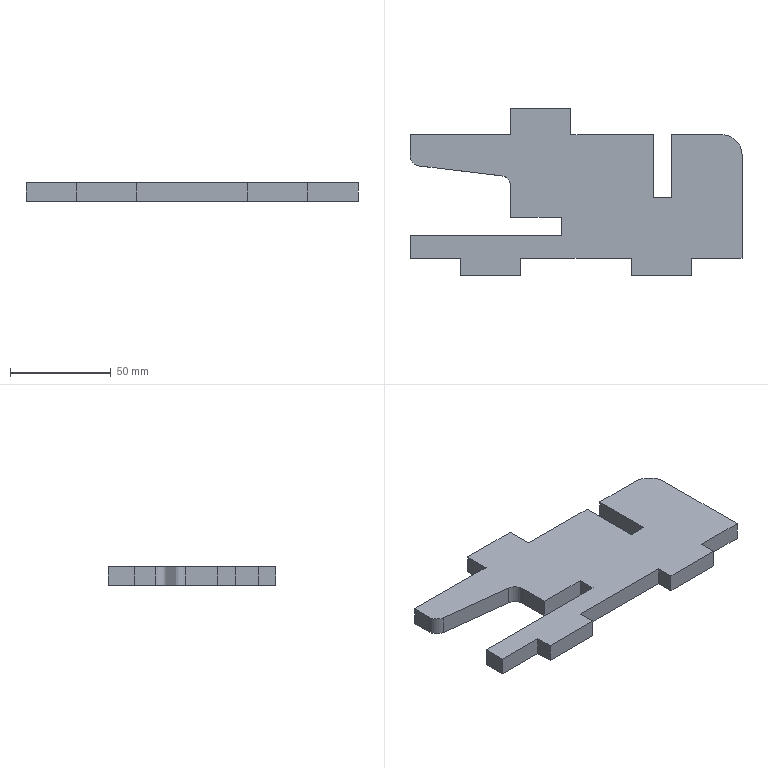Part | SolidWorks | features FlatPattern 1, SMBaseFlange 1, SheetMetal 1 | 1 solid | 31 faces | box 165 x 83 x 9 mm | volume 80282 mm3 | plane 28 | cylinder 3 | commonest cylinder face diameters 10 x2 20 x1
STEP:
#1=CARTESIAN_POINT('',(827.75,-98.803,0.));
#2=VERTEX_POINT('',#1);
#3=CARTESIAN_POINT('',(827.75,-110.303,0.));
#4=VERTEX_POINT('',#3);
#5=CARTESIAN_POINT('',(827.75,-110.303,0.));
#6=DIRECTION('',(0.,-1.,0.));
#7=VECTOR('',#6,1000.);
#8=LINE('',#5,#7);
#9=EDGE_CURVE('',#2,#4,#8,.T.);
#10=ORIENTED_EDGE('',*,*,#9,.F.);
#11=CARTESIAN_POINT('',(827.75,-98.803,-9.));
#12=VERTEX_POINT('',#11);
#13=CARTESIAN_POINT('',(827.75,-98.803,-9.));
#14=DIRECTION('',(0.,0.,1.));
#15=VECTOR('',#14,1000.);
#16=LINE('',#13,#15);
#17=EDGE_CURVE('',#12,#2,#16,.T.);
#18=ORIENTED_EDGE('',*,*,#17,.F.);
#19=CARTESIAN_POINT('',(827.75,-110.303,-9.));
#20=VERTEX_POINT('',#19);
#21=CARTESIAN_POINT('',(827.75,-110.303,-9.));
#22=DIRECTION('',(0.,-1.,0.));
#23=VECTOR('',#22,1000.);
#24=LINE('',#21,#23);
#25=EDGE_CURVE('',#12,#20,#24,.T.);
#26=ORIENTED_EDGE('',*,*,#25,.T.);
#27=CARTESIAN_POINT('',(827.75,-110.303,-9.));
#28=DIRECTION('',(0.,0.,1.));
#29=VECTOR('',#28,1000.);
#30=LINE('',#27,#29);
#31=EDGE_CURVE('',#20,#4,#30,.T.);
#32=ORIENTED_EDGE('',*,*,#31,.T.);
#33=EDGE_LOOP('',(#10,#18,#26,#32));
#34=FACE_OUTER_BOUND('',#33,.T.);
#35=CARTESIAN_POINT('',(827.75,-110.303,-9.));
#36=DIRECTION('',(-1.,0.,0.));
#37=DIRECTION('',(0.,-1.,0.));
#38=AXIS2_PLACEMENT_3D('',#35,#36,#37);
#39=PLANE('',#38);
#40=ADVANCED_FACE('',(#34),#39,.T.);
#41=CARTESIAN_POINT('',(902.95,-98.803,0.));
#42=VERTEX_POINT('',#41);
#43=CARTESIAN_POINT('',(827.75,-98.803,0.));
#44=DIRECTION('',(-1.,0.,0.));
#45=VECTOR('',#44,1000.);
#46=LINE('',#43,#45);
#47=EDGE_CURVE('',#42,#2,#46,.T.);
#48=ORIENTED_EDGE('',*,*,#47,.F.);
#49=CARTESIAN_POINT('',(902.95,-98.803,-9.));
#50=VERTEX_POINT('',#49);
#51=CARTESIAN_POINT('',(902.95,-98.803,-9.));
#52=DIRECTION('',(0.,0.,1.));
#53=VECTOR('',#52,1000.);
#54=LINE('',#51,#53);
#55=EDGE_CURVE('',#50,#42,#54,.T.);
#56=ORIENTED_EDGE('',*,*,#55,.F.);
#57=CARTESIAN_POINT('',(827.75,-98.803,-9.));
#58=DIRECTION('',(-1.,0.,0.));
#59=VECTOR('',#58,1000.);
#60=LINE('',#57,#59);
#61=EDGE_CURVE('',#50,#12,#60,.T.);
#62=ORIENTED_EDGE('',*,*,#61,.T.);
#63=ORIENTED_EDGE('',*,*,#17,.T.);
#64=EDGE_LOOP('',(#48,#56,#62,#63));
#65=FACE_OUTER_BOUND('',#64,.T.);
#66=CARTESIAN_POINT('',(827.75,-98.803,-9.));
#67=DIRECTION('',(0.,1.,0.));
#68=DIRECTION('',(0.,0.,1.));
#69=AXIS2_PLACEMENT_3D('',#66,#67,#68);
#70=PLANE('',#69);
#71=ADVANCED_FACE('',(#65),#70,.T.);
#72=CARTESIAN_POINT('',(902.95,-89.803,0.));
#73=VERTEX_POINT('',#72);
#74=CARTESIAN_POINT('',(902.95,-89.803,0.));
#75=DIRECTION('',(0.,-1.,0.));
#76=VECTOR('',#75,1000.);
#77=LINE('',#74,#76);
#78=EDGE_CURVE('',#73,#42,#77,.T.);
#79=ORIENTED_EDGE('',*,*,#78,.F.);
#80=CARTESIAN_POINT('',(902.95,-89.803,-9.));
#81=VERTEX_POINT('',#80);
#82=CARTESIAN_POINT('',(902.95,-89.803,-9.));
#83=DIRECTION('',(0.,0.,1.));
#84=VECTOR('',#83,1000.);
#85=LINE('',#82,#84);
#86=EDGE_CURVE('',#81,#73,#85,.T.);
#87=ORIENTED_EDGE('',*,*,#86,.F.);
#88=CARTESIAN_POINT('',(902.95,-89.803,-9.));
#89=DIRECTION('',(0.,-1.,0.));
#90=VECTOR('',#89,1000.);
#91=LINE('',#88,#90);
#92=EDGE_CURVE('',#81,#50,#91,.T.);
#93=ORIENTED_EDGE('',*,*,#92,.T.);
#94=ORIENTED_EDGE('',*,*,#55,.T.);
#95=EDGE_LOOP('',(#79,#87,#93,#94));
#96=FACE_OUTER_BOUND('',#95,.T.);
#97=CARTESIAN_POINT('',(902.95,-89.803,-9.));
#98=DIRECTION('',(-1.,0.,0.));
#99=DIRECTION('',(0.,0.,1.));
#100=AXIS2_PLACEMENT_3D('',#97,#98,#99);
#101=PLANE('',#100);
#102=ADVANCED_FACE('',(#96),#101,.T.);
#103=CARTESIAN_POINT('',(877.75,-89.803,0.));
#104=VERTEX_POINT('',#103);
#105=CARTESIAN_POINT('',(877.75,-89.803,0.));
#106=DIRECTION('',(1.,0.,0.));
#107=VECTOR('',#106,1000.);
#108=LINE('',#105,#107);
#109=EDGE_CURVE('',#104,#73,#108,.T.);
#110=ORIENTED_EDGE('',*,*,#109,.F.);
#111=CARTESIAN_POINT('',(877.75,-89.803,-9.));
#112=VERTEX_POINT('',#111);
#113=CARTESIAN_POINT('',(877.75,-89.803,-9.));
#114=DIRECTION('',(0.,0.,1.));
#115=VECTOR('',#114,1000.);
#116=LINE('',#113,#115);
#117=EDGE_CURVE('',#112,#104,#116,.T.);
#118=ORIENTED_EDGE('',*,*,#117,.F.);
#119=CARTESIAN_POINT('',(877.75,-89.803,-9.));
#120=DIRECTION('',(1.,0.,0.));
#121=VECTOR('',#120,1000.);
#122=LINE('',#119,#121);
#123=EDGE_CURVE('',#112,#81,#122,.T.);
#124=ORIENTED_EDGE('',*,*,#123,.T.);
#125=ORIENTED_EDGE('',*,*,#86,.T.);
#126=EDGE_LOOP('',(#110,#118,#124,#125));
#127=FACE_OUTER_BOUND('',#126,.T.);
#128=CARTESIAN_POINT('',(877.75,-89.803,-9.));
#129=DIRECTION('',(0.,-1.,0.));
#130=DIRECTION('',(1.,0.,0.));
#131=AXIS2_PLACEMENT_3D('',#128,#129,#130);
#132=PLANE('',#131);
#133=ADVANCED_FACE('',(#127),#132,.T.);
#134=CARTESIAN_POINT('',(877.75,-74.239,0.));
#135=VERTEX_POINT('',#134);
#136=CARTESIAN_POINT('',(877.75,-89.803,0.));
#137=DIRECTION('',(0.,-1.,0.));
#138=VECTOR('',#137,1000.);
#139=LINE('',#136,#138);
#140=EDGE_CURVE('',#135,#104,#139,.T.);
#141=ORIENTED_EDGE('',*,*,#140,.F.);
#142=CARTESIAN_POINT('',(877.75,-74.239,-9.));
#143=VERTEX_POINT('',#142);
#144=CARTESIAN_POINT('',(877.75,-74.239,-9.));
#145=DIRECTION('',(0.,0.,1.));
#146=VECTOR('',#145,1000.);
#147=LINE('',#144,#146);
#148=EDGE_CURVE('',#143,#135,#147,.T.);
#149=ORIENTED_EDGE('',*,*,#148,.F.);
#150=CARTESIAN_POINT('',(877.75,-89.803,-9.));
#151=DIRECTION('',(0.,-1.,0.));
#152=VECTOR('',#151,1000.);
#153=LINE('',#150,#152);
#154=EDGE_CURVE('',#143,#112,#153,.T.);
#155=ORIENTED_EDGE('',*,*,#154,.T.);
#156=ORIENTED_EDGE('',*,*,#117,.T.);
#157=EDGE_LOOP('',(#141,#149,#155,#156));
#158=FACE_OUTER_BOUND('',#157,.T.);
#159=CARTESIAN_POINT('',(877.75,-89.803,-9.));
#160=DIRECTION('',(-1.,0.,0.));
#161=DIRECTION('',(0.,-1.,0.));
#162=AXIS2_PLACEMENT_3D('',#159,#160,#161);
#163=PLANE('',#162);
#164=ADVANCED_FACE('',(#158),#163,.T.);
#165=CARTESIAN_POINT('',(873.346,-69.275,0.));
#166=VERTEX_POINT('',#165);
#167=CARTESIAN_POINT('',(872.75,-74.239,0.));
#168=DIRECTION('',(0.,0.,-1.));
#169=DIRECTION('',(1.,0.,0.));
#170=AXIS2_PLACEMENT_3D('',#167,#168,#169);
#171=CIRCLE('',#170,5.);
#172=EDGE_CURVE('',#166,#135,#171,.T.);
#173=ORIENTED_EDGE('',*,*,#172,.F.);
#174=CARTESIAN_POINT('',(873.346,-69.275,-9.));
#175=VERTEX_POINT('',#174);
#176=CARTESIAN_POINT('',(873.346,-69.275,-9.));
#177=DIRECTION('',(0.,0.,1.));
#178=VECTOR('',#177,1000.);
#179=LINE('',#176,#178);
#180=EDGE_CURVE('',#175,#166,#179,.T.);
#181=ORIENTED_EDGE('',*,*,#180,.F.);
#182=CARTESIAN_POINT('',(872.75,-74.239,-9.));
#183=DIRECTION('',(0.,0.,-1.));
#184=DIRECTION('',(1.,0.,0.));
#185=AXIS2_PLACEMENT_3D('',#182,#183,#184);
#186=CIRCLE('',#185,5.);
#187=EDGE_CURVE('',#175,#143,#186,.T.);
#188=ORIENTED_EDGE('',*,*,#187,.T.);
#189=ORIENTED_EDGE('',*,*,#148,.T.);
#190=EDGE_LOOP('',(#173,#181,#188,#189));
#191=FACE_OUTER_BOUND('',#190,.T.);
#192=CARTESIAN_POINT('',(872.75,-74.239,-9.));
#193=DIRECTION('',(0.,0.,1.));
#194=DIRECTION('',(1.,0.,0.));
#195=AXIS2_PLACEMENT_3D('',#192,#193,#194);
#196=CYLINDRICAL_SURFACE('',#195,5.);
#197=ADVANCED_FACE('',(#191),#196,.F.);
#198=CARTESIAN_POINT('',(832.154,-64.332,0.));
#199=VERTEX_POINT('',#198);
#200=CARTESIAN_POINT('',(873.346,-69.275,0.));
#201=DIRECTION('',(0.9929,-0.1191,0.));
#202=VECTOR('',#201,1000.);
#203=LINE('',#200,#202);
#204=EDGE_CURVE('',#199,#166,#203,.T.);
#205=ORIENTED_EDGE('',*,*,#204,.F.);
#206=CARTESIAN_POINT('',(832.154,-64.332,-9.));
#207=VERTEX_POINT('',#206);
#208=CARTESIAN_POINT('',(832.154,-64.332,-9.));
#209=DIRECTION('',(0.,0.,1.));
#210=VECTOR('',#209,1000.);
#211=LINE('',#208,#210);
#212=EDGE_CURVE('',#207,#199,#211,.T.);
#213=ORIENTED_EDGE('',*,*,#212,.F.);
#214=CARTESIAN_POINT('',(873.346,-69.275,-9.));
#215=DIRECTION('',(0.9929,-0.1191,0.));
#216=VECTOR('',#215,1000.);
#217=LINE('',#214,#216);
#218=EDGE_CURVE('',#207,#175,#217,.T.);
#219=ORIENTED_EDGE('',*,*,#218,.T.);
#220=ORIENTED_EDGE('',*,*,#180,.T.);
#221=EDGE_LOOP('',(#205,#213,#219,#220));
#222=FACE_OUTER_BOUND('',#221,.T.);
#223=CARTESIAN_POINT('',(873.346,-69.275,-9.));
#224=DIRECTION('',(-0.1191,-0.9929,0.));
#225=DIRECTION('',(0.9929,-0.1191,0.));
#226=AXIS2_PLACEMENT_3D('',#223,#224,#225);
#227=PLANE('',#226);
#228=ADVANCED_FACE('',(#222),#227,.T.);
#229=CARTESIAN_POINT('',(827.75,-59.367,0.));
#230=VERTEX_POINT('',#229);
#231=CARTESIAN_POINT('',(832.75,-59.367,0.));
#232=DIRECTION('',(0.,0.,1.));
#233=DIRECTION('',(-1.,0.,0.));
#234=AXIS2_PLACEMENT_3D('',#231,#232,#233);
#235=CIRCLE('',#234,5.);
#236=EDGE_CURVE('',#230,#199,#235,.T.);
#237=ORIENTED_EDGE('',*,*,#236,.F.);
#238=CARTESIAN_POINT('',(827.75,-59.367,-9.));
#239=VERTEX_POINT('',#238);
#240=CARTESIAN_POINT('',(827.75,-59.367,-9.));
#241=DIRECTION('',(0.,0.,1.));
#242=VECTOR('',#241,1000.);
#243=LINE('',#240,#242);
#244=EDGE_CURVE('',#239,#230,#243,.T.);
#245=ORIENTED_EDGE('',*,*,#244,.F.);
#246=CARTESIAN_POINT('',(832.75,-59.367,-9.));
#247=DIRECTION('',(0.,0.,1.));
#248=DIRECTION('',(-1.,0.,0.));
#249=AXIS2_PLACEMENT_3D('',#246,#247,#248);
#250=CIRCLE('',#249,5.);
#251=EDGE_CURVE('',#239,#207,#250,.T.);
#252=ORIENTED_EDGE('',*,*,#251,.T.);
#253=ORIENTED_EDGE('',*,*,#212,.T.);
#254=EDGE_LOOP('',(#237,#245,#252,#253));
#255=FACE_OUTER_BOUND('',#254,.T.);
#256=CARTESIAN_POINT('',(832.75,-59.367,-9.));
#257=DIRECTION('',(0.,0.,1.));
#258=DIRECTION('',(1.,0.,0.));
#259=AXIS2_PLACEMENT_3D('',#256,#257,#258);
#260=CYLINDRICAL_SURFACE('',#259,5.);
#261=ADVANCED_FACE('',(#255),#260,.T.);
#262=CARTESIAN_POINT('',(827.75,-48.803,0.));
#263=VERTEX_POINT('',#262);
#264=CARTESIAN_POINT('',(827.75,-48.803,0.));
#265=DIRECTION('',(0.,-1.,0.));
#266=VECTOR('',#265,1000.);
#267=LINE('',#264,#266);
#268=EDGE_CURVE('',#263,#230,#267,.T.);
#269=ORIENTED_EDGE('',*,*,#268,.F.);
#270=CARTESIAN_POINT('',(827.75,-48.803,-9.));
#271=VERTEX_POINT('',#270);
#272=CARTESIAN_POINT('',(827.75,-48.803,-9.));
#273=DIRECTION('',(0.,0.,1.));
#274=VECTOR('',#273,1000.);
#275=LINE('',#272,#274);
#276=EDGE_CURVE('',#271,#263,#275,.T.);
#277=ORIENTED_EDGE('',*,*,#276,.F.);
#278=CARTESIAN_POINT('',(827.75,-48.803,-9.));
#279=DIRECTION('',(0.,-1.,0.));
#280=VECTOR('',#279,1000.);
#281=LINE('',#278,#280);
#282=EDGE_CURVE('',#271,#239,#281,.T.);
#283=ORIENTED_EDGE('',*,*,#282,.T.);
#284=ORIENTED_EDGE('',*,*,#244,.T.);
#285=EDGE_LOOP('',(#269,#277,#283,#284));
#286=FACE_OUTER_BOUND('',#285,.T.);
#287=CARTESIAN_POINT('',(827.75,-48.803,-9.));
#288=DIRECTION('',(-1.,0.,0.));
#289=DIRECTION('',(0.,-1.,0.));
#290=AXIS2_PLACEMENT_3D('',#287,#288,#289);
#291=PLANE('',#290);
#292=ADVANCED_FACE('',(#286),#291,.T.);
#293=CARTESIAN_POINT('',(877.75,-48.803,0.));
#294=VERTEX_POINT('',#293);
#295=CARTESIAN_POINT('',(877.75,-48.803,0.));
#296=DIRECTION('',(-1.,0.,0.));
#297=VECTOR('',#296,1000.);
#298=LINE('',#295,#297);
#299=EDGE_CURVE('',#294,#263,#298,.T.);
#300=ORIENTED_EDGE('',*,*,#299,.F.);
#301=CARTESIAN_POINT('',(877.75,-48.803,-9.));
#302=VERTEX_POINT('',#301);
#303=CARTESIAN_POINT('',(877.75,-48.803,-9.));
#304=DIRECTION('',(0.,0.,1.));
#305=VECTOR('',#304,1000.);
#306=LINE('',#303,#305);
#307=EDGE_CURVE('',#302,#294,#306,.T.);
#308=ORIENTED_EDGE('',*,*,#307,.F.);
#309=CARTESIAN_POINT('',(877.75,-48.803,-9.));
#310=DIRECTION('',(-1.,0.,0.));
#311=VECTOR('',#310,1000.);
#312=LINE('',#309,#311);
#313=EDGE_CURVE('',#302,#271,#312,.T.);
#314=ORIENTED_EDGE('',*,*,#313,.T.);
#315=ORIENTED_EDGE('',*,*,#276,.T.);
#316=EDGE_LOOP('',(#300,#308,#314,#315));
#317=FACE_OUTER_BOUND('',#316,.T.);
#318=CARTESIAN_POINT('',(877.75,-48.803,-9.));
#319=DIRECTION('',(0.,1.,0.));
#320=DIRECTION('',(-1.,0.,0.));
#321=AXIS2_PLACEMENT_3D('',#318,#319,#320);
#322=PLANE('',#321);
#323=ADVANCED_FACE('',(#317),#322,.T.);
#324=CARTESIAN_POINT('',(877.75,-35.803,0.));
#325=VERTEX_POINT('',#324);
#326=CARTESIAN_POINT('',(877.75,-35.803,0.));
#327=DIRECTION('',(0.,-1.,0.));
#328=VECTOR('',#327,1000.);
#329=LINE('',#326,#328);
#330=EDGE_CURVE('',#325,#294,#329,.T.);
#331=ORIENTED_EDGE('',*,*,#330,.F.);
#332=CARTESIAN_POINT('',(877.75,-35.803,-9.));
#333=VERTEX_POINT('',#332);
#334=CARTESIAN_POINT('',(877.75,-35.803,-9.));
#335=DIRECTION('',(0.,0.,1.));
#336=VECTOR('',#335,1000.);
#337=LINE('',#334,#336);
#338=EDGE_CURVE('',#333,#325,#337,.T.);
#339=ORIENTED_EDGE('',*,*,#338,.F.);
#340=CARTESIAN_POINT('',(877.75,-35.803,-9.));
#341=DIRECTION('',(0.,-1.,0.));
#342=VECTOR('',#341,1000.);
#343=LINE('',#340,#342);
#344=EDGE_CURVE('',#333,#302,#343,.T.);
#345=ORIENTED_EDGE('',*,*,#344,.T.);
#346=ORIENTED_EDGE('',*,*,#307,.T.);
#347=EDGE_LOOP('',(#331,#339,#345,#346));
#348=FACE_OUTER_BOUND('',#347,.T.);
#349=CARTESIAN_POINT('',(877.75,-35.803,-9.));
#350=DIRECTION('',(-1.,0.,0.));
#351=DIRECTION('',(0.,0.,1.));
#352=AXIS2_PLACEMENT_3D('',#349,#350,#351);
#353=PLANE('',#352);
#354=ADVANCED_FACE('',(#348),#353,.T.);
#355=CARTESIAN_POINT('',(907.75,-35.803,0.));
#356=VERTEX_POINT('',#355);
#357=CARTESIAN_POINT('',(907.75,-35.803,0.));
#358=DIRECTION('',(-1.,0.,0.));
#359=VECTOR('',#358,1000.);
#360=LINE('',#357,#359);
#361=EDGE_CURVE('',#356,#325,#360,.T.);
#362=ORIENTED_EDGE('',*,*,#361,.F.);
#363=CARTESIAN_POINT('',(907.75,-35.803,-9.));
#364=VERTEX_POINT('',#363);
#365=CARTESIAN_POINT('',(907.75,-35.803,-9.));
#366=DIRECTION('',(0.,0.,1.));
#367=VECTOR('',#366,1000.);
#368=LINE('',#365,#367);
#369=EDGE_CURVE('',#364,#356,#368,.T.);
#370=ORIENTED_EDGE('',*,*,#369,.F.);
#371=CARTESIAN_POINT('',(907.75,-35.803,-9.));
#372=DIRECTION('',(-1.,0.,0.));
#373=VECTOR('',#372,1000.);
#374=LINE('',#371,#373);
#375=EDGE_CURVE('',#364,#333,#374,.T.);
#376=ORIENTED_EDGE('',*,*,#375,.T.);
#377=ORIENTED_EDGE('',*,*,#338,.T.);
#378=EDGE_LOOP('',(#362,#370,#376,#377));
#379=FACE_OUTER_BOUND('',#378,.T.);
#380=CARTESIAN_POINT('',(907.75,-35.803,-9.));
#381=DIRECTION('',(0.,1.,0.));
#382=DIRECTION('',(-1.,0.,0.));
#383=AXIS2_PLACEMENT_3D('',#380,#381,#382);
#384=PLANE('',#383);
#385=ADVANCED_FACE('',(#379),#384,.T.);
#386=CARTESIAN_POINT('',(907.75,-48.803,0.));
#387=VERTEX_POINT('',#386);
#388=CARTESIAN_POINT('',(907.75,-48.803,0.));
#389=DIRECTION('',(0.,1.,0.));
#390=VECTOR('',#389,1000.);
#391=LINE('',#388,#390);
#392=EDGE_CURVE('',#387,#356,#391,.T.);
#393=ORIENTED_EDGE('',*,*,#392,.F.);
#394=CARTESIAN_POINT('',(907.75,-48.803,-9.));
#395=VERTEX_POINT('',#394);
#396=CARTESIAN_POINT('',(907.75,-48.803,-9.));
#397=DIRECTION('',(0.,0.,1.));
#398=VECTOR('',#397,1000.);
#399=LINE('',#396,#398);
#400=EDGE_CURVE('',#395,#387,#399,.T.);
#401=ORIENTED_EDGE('',*,*,#400,.F.);
#402=CARTESIAN_POINT('',(907.75,-48.803,-9.));
#403=DIRECTION('',(0.,1.,0.));
#404=VECTOR('',#403,1000.);
#405=LINE('',#402,#404);
#406=EDGE_CURVE('',#395,#364,#405,.T.);
#407=ORIENTED_EDGE('',*,*,#406,.T.);
#408=ORIENTED_EDGE('',*,*,#369,.T.);
#409=EDGE_LOOP('',(#393,#401,#407,#408));
#410=FACE_OUTER_BOUND('',#409,.T.);
#411=CARTESIAN_POINT('',(907.75,-48.803,-9.));
#412=DIRECTION('',(1.,0.,0.));
#413=DIRECTION('',(0.,0.,-1.));
#414=AXIS2_PLACEMENT_3D('',#411,#412,#413);
#415=PLANE('',#414);
#416=ADVANCED_FACE('',(#410),#415,.T.);
#417=CARTESIAN_POINT('',(948.75,-48.803,0.));
#418=VERTEX_POINT('',#417);
#419=CARTESIAN_POINT('',(948.75,-48.803,0.));
#420=DIRECTION('',(-1.,0.,0.));
#421=VECTOR('',#420,1000.);
#422=LINE('',#419,#421);
#423=EDGE_CURVE('',#418,#387,#422,.T.);
#424=ORIENTED_EDGE('',*,*,#423,.F.);
#425=CARTESIAN_POINT('',(948.75,-48.803,-9.));
#426=VERTEX_POINT('',#425);
#427=CARTESIAN_POINT('',(948.75,-48.803,-9.));
#428=DIRECTION('',(0.,0.,1.));
#429=VECTOR('',#428,1000.);
#430=LINE('',#427,#429);
#431=EDGE_CURVE('',#426,#418,#430,.T.);
#432=ORIENTED_EDGE('',*,*,#431,.F.);
#433=CARTESIAN_POINT('',(948.75,-48.803,-9.));
#434=DIRECTION('',(-1.,0.,0.));
#435=VECTOR('',#434,1000.);
#436=LINE('',#433,#435);
#437=EDGE_CURVE('',#426,#395,#436,.T.);
#438=ORIENTED_EDGE('',*,*,#437,.T.);
#439=ORIENTED_EDGE('',*,*,#400,.T.);
#440=EDGE_LOOP('',(#424,#432,#438,#439));
#441=FACE_OUTER_BOUND('',#440,.T.);
#442=CARTESIAN_POINT('',(948.75,-48.803,-9.));
#443=DIRECTION('',(0.,1.,0.));
#444=DIRECTION('',(-1.,0.,0.));
#445=AXIS2_PLACEMENT_3D('',#442,#443,#444);
#446=PLANE('',#445);
#447=ADVANCED_FACE('',(#441),#446,.T.);
#448=CARTESIAN_POINT('',(948.75,-79.803,0.));
#449=VERTEX_POINT('',#448);
#450=CARTESIAN_POINT('',(948.75,-48.803,0.));
#451=DIRECTION('',(0.,1.,0.));
#452=VECTOR('',#451,1000.);
#453=LINE('',#450,#452);
#454=EDGE_CURVE('',#449,#418,#453,.T.);
#455=ORIENTED_EDGE('',*,*,#454,.F.);
#456=CARTESIAN_POINT('',(948.75,-79.803,-9.));
#457=VERTEX_POINT('',#456);
#458=CARTESIAN_POINT('',(948.75,-79.803,-9.));
#459=DIRECTION('',(0.,0.,1.));
#460=VECTOR('',#459,1000.);
#461=LINE('',#458,#460);
#462=EDGE_CURVE('',#457,#449,#461,.T.);
#463=ORIENTED_EDGE('',*,*,#462,.F.);
#464=CARTESIAN_POINT('',(948.75,-48.803,-9.));
#465=DIRECTION('',(0.,1.,0.));
#466=VECTOR('',#465,1000.);
#467=LINE('',#464,#466);
#468=EDGE_CURVE('',#457,#426,#467,.T.);
#469=ORIENTED_EDGE('',*,*,#468,.T.);
#470=ORIENTED_EDGE('',*,*,#431,.T.);
#471=EDGE_LOOP('',(#455,#463,#469,#470));
#472=FACE_OUTER_BOUND('',#471,.T.);
#473=CARTESIAN_POINT('',(948.75,-48.803,-9.));
#474=DIRECTION('',(1.,0.,0.));
#475=DIRECTION('',(0.,0.,-1.));
#476=AXIS2_PLACEMENT_3D('',#473,#474,#475);
#477=PLANE('',#476);
#478=ADVANCED_FACE('',(#472),#477,.T.);
#479=CARTESIAN_POINT('',(957.75,-79.803,0.));
#480=VERTEX_POINT('',#479);
#481=CARTESIAN_POINT('',(948.75,-79.803,0.));
#482=DIRECTION('',(-1.,0.,0.));
#483=VECTOR('',#482,1000.);
#484=LINE('',#481,#483);
#485=EDGE_CURVE('',#480,#449,#484,.T.);
#486=ORIENTED_EDGE('',*,*,#485,.F.);
#487=CARTESIAN_POINT('',(957.75,-79.803,-9.));
#488=VERTEX_POINT('',#487);
#489=CARTESIAN_POINT('',(957.75,-79.803,-9.));
#490=DIRECTION('',(0.,0.,1.));
#491=VECTOR('',#490,1000.);
#492=LINE('',#489,#491);
#493=EDGE_CURVE('',#488,#480,#492,.T.);
#494=ORIENTED_EDGE('',*,*,#493,.F.);
#495=CARTESIAN_POINT('',(948.75,-79.803,-9.));
#496=DIRECTION('',(-1.,0.,0.));
#497=VECTOR('',#496,1000.);
#498=LINE('',#495,#497);
#499=EDGE_CURVE('',#488,#457,#498,.T.);
#500=ORIENTED_EDGE('',*,*,#499,.T.);
#501=ORIENTED_EDGE('',*,*,#462,.T.);
#502=EDGE_LOOP('',(#486,#494,#500,#501));
#503=FACE_OUTER_BOUND('',#502,.T.);
#504=CARTESIAN_POINT('',(948.75,-79.803,-9.));
#505=DIRECTION('',(0.,1.,0.));
#506=DIRECTION('',(0.,0.,1.));
#507=AXIS2_PLACEMENT_3D('',#504,#505,#506);
#508=PLANE('',#507);
#509=ADVANCED_FACE('',(#503),#508,.T.);
#510=CARTESIAN_POINT('',(957.75,-48.803,0.));
#511=VERTEX_POINT('',#510);
#512=CARTESIAN_POINT('',(957.75,-79.803,0.));
#513=DIRECTION('',(0.,-1.,0.));
#514=VECTOR('',#513,1000.);
#515=LINE('',#512,#514);
#516=EDGE_CURVE('',#511,#480,#515,.T.);
#517=ORIENTED_EDGE('',*,*,#516,.F.);
#518=CARTESIAN_POINT('',(957.75,-48.803,-9.));
#519=VERTEX_POINT('',#518);
#520=CARTESIAN_POINT('',(957.75,-48.803,-9.));
#521=DIRECTION('',(0.,0.,1.));
#522=VECTOR('',#521,1000.);
#523=LINE('',#520,#522);
#524=EDGE_CURVE('',#519,#511,#523,.T.);
#525=ORIENTED_EDGE('',*,*,#524,.F.);
#526=CARTESIAN_POINT('',(957.75,-79.803,-9.));
#527=DIRECTION('',(0.,-1.,0.));
#528=VECTOR('',#527,1000.);
#529=LINE('',#526,#528);
#530=EDGE_CURVE('',#519,#488,#529,.T.);
#531=ORIENTED_EDGE('',*,*,#530,.T.);
#532=ORIENTED_EDGE('',*,*,#493,.T.);
#533=EDGE_LOOP('',(#517,#525,#531,#532));
#534=FACE_OUTER_BOUND('',#533,.T.);
#535=CARTESIAN_POINT('',(957.75,-79.803,-9.));
#536=DIRECTION('',(-1.,0.,0.));
#537=DIRECTION('',(0.,0.,1.));
#538=AXIS2_PLACEMENT_3D('',#535,#536,#537);
#539=PLANE('',#538);
#540=ADVANCED_FACE('',(#534),#539,.T.);
#541=CARTESIAN_POINT('',(982.75,-48.803,0.));
#542=VERTEX_POINT('',#541);
#543=CARTESIAN_POINT('',(982.75,-48.803,0.));
#544=DIRECTION('',(-1.,0.,0.));
#545=VECTOR('',#544,1000.);
#546=LINE('',#543,#545);
#547=EDGE_CURVE('',#542,#511,#546,.T.);
#548=ORIENTED_EDGE('',*,*,#547,.F.);
#549=CARTESIAN_POINT('',(982.75,-48.803,-9.));
#550=VERTEX_POINT('',#549);
#551=CARTESIAN_POINT('',(982.75,-48.803,-9.));
#552=DIRECTION('',(0.,0.,1.));
#553=VECTOR('',#552,1000.);
#554=LINE('',#551,#553);
#555=EDGE_CURVE('',#550,#542,#554,.T.);
#556=ORIENTED_EDGE('',*,*,#555,.F.);
#557=CARTESIAN_POINT('',(982.75,-48.803,-9.));
#558=DIRECTION('',(-1.,0.,0.));
#559=VECTOR('',#558,1000.);
#560=LINE('',#557,#559);
#561=EDGE_CURVE('',#550,#519,#560,.T.);
#562=ORIENTED_EDGE('',*,*,#561,.T.);
#563=ORIENTED_EDGE('',*,*,#524,.T.);
#564=EDGE_LOOP('',(#548,#556,#562,#563));
#565=FACE_OUTER_BOUND('',#564,.T.);
#566=CARTESIAN_POINT('',(982.75,-48.803,-9.));
#567=DIRECTION('',(0.,1.,0.));
#568=DIRECTION('',(-1.,0.,0.));
#569=AXIS2_PLACEMENT_3D('',#566,#567,#568);
#570=PLANE('',#569);
#571=ADVANCED_FACE('',(#565),#570,.T.);
#572=CARTESIAN_POINT('',(992.75,-58.803,0.));
#573=VERTEX_POINT('',#572);
#574=CARTESIAN_POINT('',(982.75,-58.803,0.));
#575=DIRECTION('',(0.,0.,1.));
#576=DIRECTION('',(1.,0.,0.));
#577=AXIS2_PLACEMENT_3D('',#574,#575,#576);
#578=CIRCLE('',#577,10.);
#579=EDGE_CURVE('',#573,#542,#578,.T.);
#580=ORIENTED_EDGE('',*,*,#579,.F.);
#581=CARTESIAN_POINT('',(992.75,-58.803,-9.));
#582=VERTEX_POINT('',#581);
#583=CARTESIAN_POINT('',(992.75,-58.803,-9.));
#584=DIRECTION('',(0.,0.,1.));
#585=VECTOR('',#584,1000.);
#586=LINE('',#583,#585);
#587=EDGE_CURVE('',#582,#573,#586,.T.);
#588=ORIENTED_EDGE('',*,*,#587,.F.);
#589=CARTESIAN_POINT('',(982.75,-58.803,-9.));
#590=DIRECTION('',(0.,0.,1.));
#591=DIRECTION('',(1.,0.,0.));
#592=AXIS2_PLACEMENT_3D('',#589,#590,#591);
#593=CIRCLE('',#592,10.);
#594=EDGE_CURVE('',#582,#550,#593,.T.);
#595=ORIENTED_EDGE('',*,*,#594,.T.);
#596=ORIENTED_EDGE('',*,*,#555,.T.);
#597=EDGE_LOOP('',(#580,#588,#595,#596));
#598=FACE_OUTER_BOUND('',#597,.T.);
#599=CARTESIAN_POINT('',(982.75,-58.803,-9.));
#600=DIRECTION('',(0.,0.,1.));
#601=DIRECTION('',(1.,0.,0.));
#602=AXIS2_PLACEMENT_3D('',#599,#600,#601);
#603=CYLINDRICAL_SURFACE('',#602,10.);
#604=ADVANCED_FACE('',(#598),#603,.T.);
#605=CARTESIAN_POINT('',(992.75,-110.303,0.));
#606=VERTEX_POINT('',#605);
#607=CARTESIAN_POINT('',(992.75,-110.303,0.));
#608=DIRECTION('',(0.,1.,0.));
#609=VECTOR('',#608,1000.);
#610=LINE('',#607,#609);
#611=EDGE_CURVE('',#606,#573,#610,.T.);
#612=ORIENTED_EDGE('',*,*,#611,.F.);
#613=CARTESIAN_POINT('',(992.75,-110.303,-9.));
#614=VERTEX_POINT('',#613);
#615=CARTESIAN_POINT('',(992.75,-110.303,-9.));
#616=DIRECTION('',(0.,0.,1.));
#617=VECTOR('',#616,1000.);
#618=LINE('',#615,#617);
#619=EDGE_CURVE('',#614,#606,#618,.T.);
#620=ORIENTED_EDGE('',*,*,#619,.F.);
#621=CARTESIAN_POINT('',(992.75,-110.303,-9.));
#622=DIRECTION('',(0.,1.,0.));
#623=VECTOR('',#622,1000.);
#624=LINE('',#621,#623);
#625=EDGE_CURVE('',#614,#582,#624,.T.);
#626=ORIENTED_EDGE('',*,*,#625,.T.);
#627=ORIENTED_EDGE('',*,*,#587,.T.);
#628=EDGE_LOOP('',(#612,#620,#626,#627));
#629=FACE_OUTER_BOUND('',#628,.T.);
#630=CARTESIAN_POINT('',(992.75,-110.303,-9.));
#631=DIRECTION('',(1.,0.,0.));
#632=DIRECTION('',(0.,0.,-1.));
#633=AXIS2_PLACEMENT_3D('',#630,#631,#632);
#634=PLANE('',#633);
#635=ADVANCED_FACE('',(#629),#634,.T.);
#636=CARTESIAN_POINT('',(967.75,-110.303,0.));
#637=VERTEX_POINT('',#636);
#638=CARTESIAN_POINT('',(967.75,-110.303,0.));
#639=DIRECTION('',(1.,0.,0.));
#640=VECTOR('',#639,1000.);
#641=LINE('',#638,#640);
#642=EDGE_CURVE('',#637,#606,#641,.T.);
#643=ORIENTED_EDGE('',*,*,#642,.F.);
#644=CARTESIAN_POINT('',(967.75,-110.303,-9.));
#645=VERTEX_POINT('',#644);
#646=CARTESIAN_POINT('',(967.75,-110.303,-9.));
#647=DIRECTION('',(0.,0.,1.));
#648=VECTOR('',#647,1000.);
#649=LINE('',#646,#648);
#650=EDGE_CURVE('',#645,#637,#649,.T.);
#651=ORIENTED_EDGE('',*,*,#650,.F.);
#652=CARTESIAN_POINT('',(967.75,-110.303,-9.));
#653=DIRECTION('',(1.,0.,0.));
#654=VECTOR('',#653,1000.);
#655=LINE('',#652,#654);
#656=EDGE_CURVE('',#645,#614,#655,.T.);
#657=ORIENTED_EDGE('',*,*,#656,.T.);
#658=ORIENTED_EDGE('',*,*,#619,.T.);
#659=EDGE_LOOP('',(#643,#651,#657,#658));
#660=FACE_OUTER_BOUND('',#659,.T.);
#661=CARTESIAN_POINT('',(967.75,-110.303,-9.));
#662=DIRECTION('',(0.,-1.,0.));
#663=DIRECTION('',(1.,0.,0.));
#664=AXIS2_PLACEMENT_3D('',#661,#662,#663);
#665=PLANE('',#664);
#666=ADVANCED_FACE('',(#660),#665,.T.);
#667=CARTESIAN_POINT('',(967.75,-118.803,0.));
#668=VERTEX_POINT('',#667);
#669=CARTESIAN_POINT('',(967.75,-118.803,0.));
#670=DIRECTION('',(0.,1.,0.));
#671=VECTOR('',#670,1000.);
#672=LINE('',#669,#671);
#673=EDGE_CURVE('',#668,#637,#672,.T.);
#674=ORIENTED_EDGE('',*,*,#673,.F.);
#675=CARTESIAN_POINT('',(967.75,-118.803,-9.));
#676=VERTEX_POINT('',#675);
#677=CARTESIAN_POINT('',(967.75,-118.803,-9.));
#678=DIRECTION('',(0.,0.,1.));
#679=VECTOR('',#678,1000.);
#680=LINE('',#677,#679);
#681=EDGE_CURVE('',#676,#668,#680,.T.);
#682=ORIENTED_EDGE('',*,*,#681,.F.);
#683=CARTESIAN_POINT('',(967.75,-118.803,-9.));
#684=DIRECTION('',(0.,1.,0.));
#685=VECTOR('',#684,1000.);
#686=LINE('',#683,#685);
#687=EDGE_CURVE('',#676,#645,#686,.T.);
#688=ORIENTED_EDGE('',*,*,#687,.T.);
#689=ORIENTED_EDGE('',*,*,#650,.T.);
#690=EDGE_LOOP('',(#674,#682,#688,#689));
#691=FACE_OUTER_BOUND('',#690,.T.);
#692=CARTESIAN_POINT('',(967.75,-118.803,-9.));
#693=DIRECTION('',(1.,0.,0.));
#694=DIRECTION('',(0.,0.,-1.));
#695=AXIS2_PLACEMENT_3D('',#692,#693,#694);
#696=PLANE('',#695);
#697=ADVANCED_FACE('',(#691),#696,.T.);
#698=CARTESIAN_POINT('',(937.75,-118.803,0.));
#699=VERTEX_POINT('',#698);
#700=CARTESIAN_POINT('',(937.75,-118.803,0.));
#701=DIRECTION('',(1.,0.,0.));
#702=VECTOR('',#701,1000.);
#703=LINE('',#700,#702);
#704=EDGE_CURVE('',#699,#668,#703,.T.);
#705=ORIENTED_EDGE('',*,*,#704,.F.);
#706=CARTESIAN_POINT('',(937.75,-118.803,-9.));
#707=VERTEX_POINT('',#706);
#708=CARTESIAN_POINT('',(937.75,-118.803,-9.));
#709=DIRECTION('',(0.,0.,1.));
#710=VECTOR('',#709,1000.);
#711=LINE('',#708,#710);
#712=EDGE_CURVE('',#707,#699,#711,.T.);
#713=ORIENTED_EDGE('',*,*,#712,.F.);
#714=CARTESIAN_POINT('',(937.75,-118.803,-9.));
#715=DIRECTION('',(1.,0.,0.));
#716=VECTOR('',#715,1000.);
#717=LINE('',#714,#716);
#718=EDGE_CURVE('',#707,#676,#717,.T.);
#719=ORIENTED_EDGE('',*,*,#718,.T.);
#720=ORIENTED_EDGE('',*,*,#681,.T.);
#721=EDGE_LOOP('',(#705,#713,#719,#720));
#722=FACE_OUTER_BOUND('',#721,.T.);
#723=CARTESIAN_POINT('',(937.75,-118.803,-9.));
#724=DIRECTION('',(0.,-1.,0.));
#725=DIRECTION('',(0.,0.,-1.));
#726=AXIS2_PLACEMENT_3D('',#723,#724,#725);
#727=PLANE('',#726);
#728=ADVANCED_FACE('',(#722),#727,.T.);
#729=CARTESIAN_POINT('',(937.75,-110.303,0.));
#730=VERTEX_POINT('',#729);
#731=CARTESIAN_POINT('',(937.75,-110.303,0.));
#732=DIRECTION('',(0.,-1.,0.));
#733=VECTOR('',#732,1000.);
#734=LINE('',#731,#733);
#735=EDGE_CURVE('',#730,#699,#734,.T.);
#736=ORIENTED_EDGE('',*,*,#735,.F.);
#737=CARTESIAN_POINT('',(937.75,-110.303,-9.));
#738=VERTEX_POINT('',#737);
#739=CARTESIAN_POINT('',(937.75,-110.303,-9.));
#740=DIRECTION('',(0.,0.,1.));
#741=VECTOR('',#740,1000.);
#742=LINE('',#739,#741);
#743=EDGE_CURVE('',#738,#730,#742,.T.);
#744=ORIENTED_EDGE('',*,*,#743,.F.);
#745=CARTESIAN_POINT('',(937.75,-110.303,-9.));
#746=DIRECTION('',(0.,-1.,0.));
#747=VECTOR('',#746,1000.);
#748=LINE('',#745,#747);
#749=EDGE_CURVE('',#738,#707,#748,.T.);
#750=ORIENTED_EDGE('',*,*,#749,.T.);
#751=ORIENTED_EDGE('',*,*,#712,.T.);
#752=EDGE_LOOP('',(#736,#744,#750,#751));
#753=FACE_OUTER_BOUND('',#752,.T.);
#754=CARTESIAN_POINT('',(937.75,-110.303,-9.));
#755=DIRECTION('',(-1.,0.,0.));
#756=DIRECTION('',(0.,0.,1.));
#757=AXIS2_PLACEMENT_3D('',#754,#755,#756);
#758=PLANE('',#757);
#759=ADVANCED_FACE('',(#753),#758,.T.);
#760=CARTESIAN_POINT('',(882.75,-110.303,0.));
#761=VERTEX_POINT('',#760);
#762=CARTESIAN_POINT('',(882.75,-110.303,0.));
#763=DIRECTION('',(1.,0.,0.));
#764=VECTOR('',#763,1000.);
#765=LINE('',#762,#764);
#766=EDGE_CURVE('',#761,#730,#765,.T.);
#767=ORIENTED_EDGE('',*,*,#766,.F.);
#768=CARTESIAN_POINT('',(882.75,-110.303,-9.));
#769=VERTEX_POINT('',#768);
#770=CARTESIAN_POINT('',(882.75,-110.303,-9.));
#771=DIRECTION('',(0.,0.,1.));
#772=VECTOR('',#771,1000.);
#773=LINE('',#770,#772);
#774=EDGE_CURVE('',#769,#761,#773,.T.);
#775=ORIENTED_EDGE('',*,*,#774,.F.);
#776=CARTESIAN_POINT('',(882.75,-110.303,-9.));
#777=DIRECTION('',(1.,0.,0.));
#778=VECTOR('',#777,1000.);
#779=LINE('',#776,#778);
#780=EDGE_CURVE('',#769,#738,#779,.T.);
#781=ORIENTED_EDGE('',*,*,#780,.T.);
#782=ORIENTED_EDGE('',*,*,#743,.T.);
#783=EDGE_LOOP('',(#767,#775,#781,#782));
#784=FACE_OUTER_BOUND('',#783,.T.);
#785=CARTESIAN_POINT('',(882.75,-110.303,-9.));
#786=DIRECTION('',(0.,-1.,0.));
#787=DIRECTION('',(0.,0.,-1.));
#788=AXIS2_PLACEMENT_3D('',#785,#786,#787);
#789=PLANE('',#788);
#790=ADVANCED_FACE('',(#784),#789,.T.);
#791=CARTESIAN_POINT('',(882.75,-118.803,0.));
#792=VERTEX_POINT('',#791);
#793=CARTESIAN_POINT('',(882.75,-118.803,0.));
#794=DIRECTION('',(0.,1.,0.));
#795=VECTOR('',#794,1000.);
#796=LINE('',#793,#795);
#797=EDGE_CURVE('',#792,#761,#796,.T.);
#798=ORIENTED_EDGE('',*,*,#797,.F.);
#799=CARTESIAN_POINT('',(882.75,-118.803,-9.));
#800=VERTEX_POINT('',#799);
#801=CARTESIAN_POINT('',(882.75,-118.803,-9.));
#802=DIRECTION('',(0.,0.,1.));
#803=VECTOR('',#802,1000.);
#804=LINE('',#801,#803);
#805=EDGE_CURVE('',#800,#792,#804,.T.);
#806=ORIENTED_EDGE('',*,*,#805,.F.);
#807=CARTESIAN_POINT('',(882.75,-118.803,-9.));
#808=DIRECTION('',(0.,1.,0.));
#809=VECTOR('',#808,1000.);
#810=LINE('',#807,#809);
#811=EDGE_CURVE('',#800,#769,#810,.T.);
#812=ORIENTED_EDGE('',*,*,#811,.T.);
#813=ORIENTED_EDGE('',*,*,#774,.T.);
#814=EDGE_LOOP('',(#798,#806,#812,#813));
#815=FACE_OUTER_BOUND('',#814,.T.);
#816=CARTESIAN_POINT('',(882.75,-118.803,-9.));
#817=DIRECTION('',(1.,0.,0.));
#818=DIRECTION('',(0.,0.,-1.));
#819=AXIS2_PLACEMENT_3D('',#816,#817,#818);
#820=PLANE('',#819);
#821=ADVANCED_FACE('',(#815),#820,.T.);
#822=CARTESIAN_POINT('',(852.75,-118.803,0.));
#823=VERTEX_POINT('',#822);
#824=CARTESIAN_POINT('',(852.75,-118.803,0.));
#825=DIRECTION('',(1.,0.,0.));
#826=VECTOR('',#825,1000.);
#827=LINE('',#824,#826);
#828=EDGE_CURVE('',#823,#792,#827,.T.);
#829=ORIENTED_EDGE('',*,*,#828,.F.);
#830=CARTESIAN_POINT('',(852.75,-118.803,-9.));
#831=VERTEX_POINT('',#830);
#832=CARTESIAN_POINT('',(852.75,-118.803,-9.));
#833=DIRECTION('',(0.,0.,1.));
#834=VECTOR('',#833,1000.);
#835=LINE('',#832,#834);
#836=EDGE_CURVE('',#831,#823,#835,.T.);
#837=ORIENTED_EDGE('',*,*,#836,.F.);
#838=CARTESIAN_POINT('',(852.75,-118.803,-9.));
#839=DIRECTION('',(1.,0.,0.));
#840=VECTOR('',#839,1000.);
#841=LINE('',#838,#840);
#842=EDGE_CURVE('',#831,#800,#841,.T.);
#843=ORIENTED_EDGE('',*,*,#842,.T.);
#844=ORIENTED_EDGE('',*,*,#805,.T.);
#845=EDGE_LOOP('',(#829,#837,#843,#844));
#846=FACE_OUTER_BOUND('',#845,.T.);
#847=CARTESIAN_POINT('',(852.75,-118.803,-9.));
#848=DIRECTION('',(0.,-1.,0.));
#849=DIRECTION('',(0.,0.,-1.));
#850=AXIS2_PLACEMENT_3D('',#847,#848,#849);
#851=PLANE('',#850);
#852=ADVANCED_FACE('',(#846),#851,.T.);
#853=CARTESIAN_POINT('',(852.75,-110.303,0.));
#854=VERTEX_POINT('',#853);
#855=CARTESIAN_POINT('',(852.75,-110.303,0.));
#856=DIRECTION('',(0.,-1.,0.));
#857=VECTOR('',#856,1000.);
#858=LINE('',#855,#857);
#859=EDGE_CURVE('',#854,#823,#858,.T.);
#860=ORIENTED_EDGE('',*,*,#859,.F.);
#861=CARTESIAN_POINT('',(852.75,-110.303,-9.));
#862=VERTEX_POINT('',#861);
#863=CARTESIAN_POINT('',(852.75,-110.303,-9.));
#864=DIRECTION('',(0.,0.,1.));
#865=VECTOR('',#864,1000.);
#866=LINE('',#863,#865);
#867=EDGE_CURVE('',#862,#854,#866,.T.);
#868=ORIENTED_EDGE('',*,*,#867,.F.);
#869=CARTESIAN_POINT('',(852.75,-110.303,-9.));
#870=DIRECTION('',(0.,-1.,0.));
#871=VECTOR('',#870,1000.);
#872=LINE('',#869,#871);
#873=EDGE_CURVE('',#862,#831,#872,.T.);
#874=ORIENTED_EDGE('',*,*,#873,.T.);
#875=ORIENTED_EDGE('',*,*,#836,.T.);
#876=EDGE_LOOP('',(#860,#868,#874,#875));
#877=FACE_OUTER_BOUND('',#876,.T.);
#878=CARTESIAN_POINT('',(852.75,-110.303,-9.));
#879=DIRECTION('',(-1.,0.,0.));
#880=DIRECTION('',(0.,-1.,0.));
#881=AXIS2_PLACEMENT_3D('',#878,#879,#880);
#882=PLANE('',#881);
#883=ADVANCED_FACE('',(#877),#882,.T.);
#884=CARTESIAN_POINT('',(827.75,-110.303,0.));
#885=DIRECTION('',(1.,0.,0.));
#886=VECTOR('',#885,1000.);
#887=LINE('',#884,#886);
#888=EDGE_CURVE('',#4,#854,#887,.T.);
#889=ORIENTED_EDGE('',*,*,#888,.F.);
#890=ORIENTED_EDGE('',*,*,#31,.F.);
#891=CARTESIAN_POINT('',(827.75,-110.303,-9.));
#892=DIRECTION('',(1.,0.,0.));
#893=VECTOR('',#892,1000.);
#894=LINE('',#891,#893);
#895=EDGE_CURVE('',#20,#862,#894,.T.);
#896=ORIENTED_EDGE('',*,*,#895,.T.);
#897=ORIENTED_EDGE('',*,*,#867,.T.);
#898=EDGE_LOOP('',(#889,#890,#896,#897));
#899=FACE_OUTER_BOUND('',#898,.T.);
#900=CARTESIAN_POINT('',(827.75,-110.303,-9.));
#901=DIRECTION('',(0.,-1.,0.));
#902=DIRECTION('',(1.,0.,0.));
#903=AXIS2_PLACEMENT_3D('',#900,#901,#902);
#904=PLANE('',#903);
#905=ADVANCED_FACE('',(#899),#904,.T.);
#906=ORIENTED_EDGE('',*,*,#25,.F.);
#907=ORIENTED_EDGE('',*,*,#61,.F.);
#908=ORIENTED_EDGE('',*,*,#92,.F.);
#909=ORIENTED_EDGE('',*,*,#123,.F.);
#910=ORIENTED_EDGE('',*,*,#154,.F.);
#911=ORIENTED_EDGE('',*,*,#187,.F.);
#912=ORIENTED_EDGE('',*,*,#218,.F.);
#913=ORIENTED_EDGE('',*,*,#251,.F.);
#914=ORIENTED_EDGE('',*,*,#282,.F.);
#915=ORIENTED_EDGE('',*,*,#313,.F.);
#916=ORIENTED_EDGE('',*,*,#344,.F.);
#917=ORIENTED_EDGE('',*,*,#375,.F.);
#918=ORIENTED_EDGE('',*,*,#406,.F.);
#919=ORIENTED_EDGE('',*,*,#437,.F.);
#920=ORIENTED_EDGE('',*,*,#468,.F.);
#921=ORIENTED_EDGE('',*,*,#499,.F.);
#922=ORIENTED_EDGE('',*,*,#530,.F.);
#923=ORIENTED_EDGE('',*,*,#561,.F.);
#924=ORIENTED_EDGE('',*,*,#594,.F.);
#925=ORIENTED_EDGE('',*,*,#625,.F.);
#926=ORIENTED_EDGE('',*,*,#656,.F.);
#927=ORIENTED_EDGE('',*,*,#687,.F.);
#928=ORIENTED_EDGE('',*,*,#718,.F.);
#929=ORIENTED_EDGE('',*,*,#749,.F.);
#930=ORIENTED_EDGE('',*,*,#780,.F.);
#931=ORIENTED_EDGE('',*,*,#811,.F.);
#932=ORIENTED_EDGE('',*,*,#842,.F.);
#933=ORIENTED_EDGE('',*,*,#873,.F.);
#934=ORIENTED_EDGE('',*,*,#895,.F.);
#935=EDGE_LOOP('',(#906,#907,#908,#909,#910,#911,#912,#913,#914,#915,#916,#917,#918,#919,#920,#921,#922,#923,#924,#925,#926,#927,#928,#929,#930,#931,#932,#933,#934));
#936=FACE_OUTER_BOUND('',#935,.T.);
#937=CARTESIAN_POINT('',(872.75,-74.239,-9.));
#938=DIRECTION('',(0.,0.,1.));
#939=DIRECTION('',(1.,0.,0.));
#940=AXIS2_PLACEMENT_3D('',#937,#938,#939);
#941=PLANE('',#940);
#942=ADVANCED_FACE('',(#936),#941,.F.);
#943=ORIENTED_EDGE('',*,*,#9,.T.);
#944=ORIENTED_EDGE('',*,*,#888,.T.);
#945=ORIENTED_EDGE('',*,*,#859,.T.);
#946=ORIENTED_EDGE('',*,*,#828,.T.);
#947=ORIENTED_EDGE('',*,*,#797,.T.);
#948=ORIENTED_EDGE('',*,*,#766,.T.);
#949=ORIENTED_EDGE('',*,*,#735,.T.);
#950=ORIENTED_EDGE('',*,*,#704,.T.);
#951=ORIENTED_EDGE('',*,*,#673,.T.);
#952=ORIENTED_EDGE('',*,*,#642,.T.);
#953=ORIENTED_EDGE('',*,*,#611,.T.);
#954=ORIENTED_EDGE('',*,*,#579,.T.);
#955=ORIENTED_EDGE('',*,*,#547,.T.);
#956=ORIENTED_EDGE('',*,*,#516,.T.);
#957=ORIENTED_EDGE('',*,*,#485,.T.);
#958=ORIENTED_EDGE('',*,*,#454,.T.);
#959=ORIENTED_EDGE('',*,*,#423,.T.);
#960=ORIENTED_EDGE('',*,*,#392,.T.);
#961=ORIENTED_EDGE('',*,*,#361,.T.);
#962=ORIENTED_EDGE('',*,*,#330,.T.);
#963=ORIENTED_EDGE('',*,*,#299,.T.);
#964=ORIENTED_EDGE('',*,*,#268,.T.);
#965=ORIENTED_EDGE('',*,*,#236,.T.);
#966=ORIENTED_EDGE('',*,*,#204,.T.);
#967=ORIENTED_EDGE('',*,*,#172,.T.);
#968=ORIENTED_EDGE('',*,*,#140,.T.);
#969=ORIENTED_EDGE('',*,*,#109,.T.);
#970=ORIENTED_EDGE('',*,*,#78,.T.);
#971=ORIENTED_EDGE('',*,*,#47,.T.);
#972=EDGE_LOOP('',(#943,#944,#945,#946,#947,#948,#949,#950,#951,#952,#953,#954,#955,#956,#957,#958,#959,#960,#961,#962,#963,#964,#965,#966,#967,#968,#969,#970,#971));
#973=FACE_OUTER_BOUND('',#972,.T.);
#974=CARTESIAN_POINT('',(872.75,-74.239,0.));
#975=DIRECTION('',(0.,0.,1.));
#976=DIRECTION('',(1.,0.,0.));
#977=AXIS2_PLACEMENT_3D('',#974,#975,#976);
#978=PLANE('',#977);
#979=ADVANCED_FACE('',(#973),#978,.T.);
#980=CLOSED_SHELL('',(#40,#71,#102,#133,#164,#197,#228,#261,#292,#323,#354,#385,#416,#447,#478,#509,#540,#571,#604,#635,#666,#697,#728,#759,#790,#821,#852,#883,#905,#942,#979));
#981=MANIFOLD_SOLID_BREP('',#980);
#982=CARTESIAN_POINT('',(0.,0.,0.));
#983=DIRECTION('',(0.,0.,1.));
#984=DIRECTION('',(1.,0.,0.));
#985=AXIS2_PLACEMENT_3D('',#982,#983,#984);
#986=(LENGTH_UNIT()NAMED_UNIT(*)SI_UNIT(.MILLI.,.METRE.));
#987=UNCERTAINTY_MEASURE_WITH_UNIT(LENGTH_MEASURE(0.00001),#986,'','');
#988=(NAMED_UNIT(*)PLANE_ANGLE_UNIT()SI_UNIT($,.RADIAN.));
#989=(NAMED_UNIT(*)SI_UNIT($,.STERADIAN.)SOLID_ANGLE_UNIT());
#990=(GEOMETRIC_REPRESENTATION_CONTEXT(3)GLOBAL_UNCERTAINTY_ASSIGNED_CONTEXT((#987))GLOBAL_UNIT_ASSIGNED_CONTEXT((#986,#988,#989))REPRESENTATION_CONTEXT('',''));
#991=ADVANCED_BREP_SHAPE_REPRESENTATION('',(#981,#985),#990);